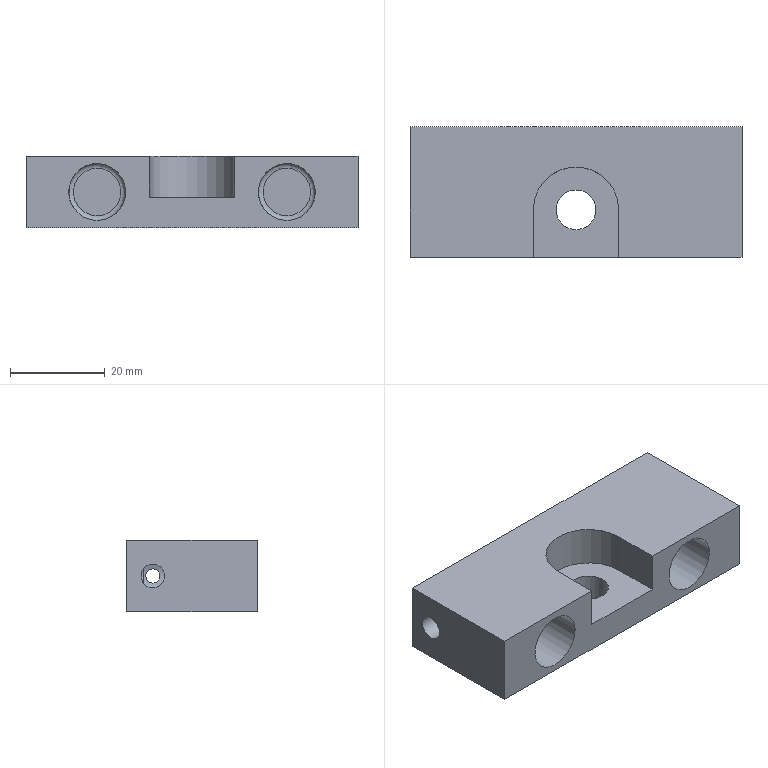NC program | NX | posted with a generic post | part box 70 x 27.5 x 15 mm
Lines 3562 to 3781 of 3781:
(PLANAR_MILL_8_COPY , TOOL : D8R1)
N7098 T04 M6
N7100 G54
N7102 G17 G0 G90 X-19.087 Y1.24 B0. C0. S2500 M3
N7104 G43 Z20. H4
N7106 Z-5.983 B-180. C-180.
N7108 G94 G1 Z-7.983 F300.
N7110 G41 X-19. Y1.732 D4
N7112 Y2.
N7114 G3 X-20. Y3. R1.
N7116 X-23. Y0. R3.
N7118 X-20. Y3. R-3.
N7120 X-21. Y2. R1.
N7122 G40
N7124 G1 X-20.913 Y1.508
N7126 X-19.087
N7128 G41 X-19. Y2.
N7130 G3 X-20. Y3. R1.
N7132 X-23. Y0. R3.
N7134 X-20. Y3. R-3.
N7136 X-21. Y2. R1.
N7138 G1 Y1.732
N7140 G40
N7142 X-20.913 Y1.24
N7144 Z-5.983
N7146 G0 Z20.
N7148 X-19.087
N7150 Z-13.967
N7152 G1 Z-15.967
N7154 G41 X-19. Y1.732
N7156 Y2.
N7158 G3 X-20. Y3. R1.
N7160 X-23. Y0. R3.
N7162 X-20. Y3. R-3.
N7164 X-21. Y2. R1.
N7166 G40
N7168 G1 X-20.913 Y1.508
N7170 X-19.087
N7172 G41 X-19. Y2.
N7174 G3 X-20. Y3. R1.
N7176 X-23. Y0. R3.
N7178 X-20. Y3. R-3.
N7180 X-21. Y2. R1.
N7182 G1 Y1.732
N7184 G40
N7186 X-20.913 Y1.24
N7188 Z-13.967
N7190 G0 Z20.
N7192 X-19.087
N7194 Z-21.95
N7196 G1 Z-23.95
N7198 G41 X-19. Y1.732
N7200 Y2.
N7202 G3 X-20. Y3. R1.
N7204 X-23. Y0. R3.
N7206 X-20. Y3. R-3.
N7208 X-21. Y2. R1.
N7210 G40
N7212 G1 X-20.913 Y1.508
N7214 X-19.087
N7216 G41 X-19. Y2.
N7218 G3 X-20. Y3. R1.
N7220 X-23. Y0. R3.
N7222 X-20. Y3. R-3.
N7224 X-21. Y2. R1.
N7226 G1 Y1.732
N7228 G40
N7230 X-20.913 Y1.24
N7232 Z-21.95
N7234 G0 Z20.
N7236 X20.913
N7238 Z-5.983
N7240 G1 Z-7.983
N7242 G41 X21. Y1.732
N7244 Y2.
N7246 G3 X20. Y3. R1.
N7248 X17. Y0. R3.
N7250 X20. Y3. R-3.
N7252 X19. Y2. R1.
N7254 G40
N7256 G1 X19.087 Y1.508
N7258 X20.913
N7260 G41 X21. Y2.
N7262 G3 X20. Y3. R1.
N7264 X17. Y0. R3.
N7266 X20. Y3. R-3.
N7268 X19. Y2. R1.
N7270 G1 Y1.732
N7272 G40
N7274 X19.087 Y1.24
N7276 Z-5.983
N7278 G0 Z20.
N7280 X20.913
N7282 Z-13.967
N7284 G1 Z-15.967
N7286 G41 X21. Y1.732
N7288 Y2.
N7290 G3 X20. Y3. R1.
N7292 X17. Y0. R3.
N7294 X20. Y3. R-3.
N7296 X19. Y2. R1.
N7298 G40
N7300 G1 X19.087 Y1.508
N7302 X20.913
N7304 G41 X21. Y2.
N7306 G3 X20. Y3. R1.
N7308 X17. Y0. R3.
N7310 X20. Y3. R-3.
N7312 X19. Y2. R1.
N7314 G1 Y1.732
N7316 G40
N7318 X19.087 Y1.24
N7320 Z-13.967
N7322 G0 Z20.
N7324 X20.913
N7326 Z-21.95
N7328 G1 Z-23.95
N7330 G41 X21. Y1.732
N7332 Y2.
N7334 G3 X20. Y3. R1.
N7336 X17. Y0. R3.
N7338 X20. Y3. R-3.
N7340 X19. Y2. R1.
N7342 G40
N7344 G1 X19.087 Y1.508
N7346 X20.913
N7348 G41 X21. Y2.
N7350 G3 X20. Y3. R1.
N7352 X17. Y0. R3.
N7354 X20. Y3. R-3.
N7356 X19. Y2. R1.
N7358 G1 Y1.732
N7360 G40
N7362 X19.087 Y1.24
N7364 Z-21.95
N7366 G0 Z20.
(PLANAR_MILL_9 , TOOL : D8R1)
N7368 X-19.629 Y0.149 S3000
N7370 Z-23.
N7372 G1 Z-25.
N7374 G41 X-19. Y0.4
N7376 G3 X-20. Y1.4 R1.
N7378 X-21.4 Y0. R1.4
N7380 X-20. Y1.4 R-1.4
N7382 X-21. Y0.4 R1.
N7384 G40
N7386 G1 X-20.983 Y0.302
N7388 X-19.017 Y1.902
N7390 G41 X-19. Y2.
N7392 G3 X-20. Y3. R1.
N7394 X-23. Y0. R3.
N7396 X-20. Y3. R-3.
N7398 X-21. Y2. R1.
N7400 G1 Y1.732
N7402 G40
N7404 X-20.983 Y1.634
N7406 Z-23.
N7408 G0 Z20.
N7410 X20.371 Y0.149
N7412 Z-23.
N7414 G1 Z-25.
N7416 G41 X21. Y0.4
N7418 G3 X20. Y1.4 R1.
N7420 X18.6 Y0. R1.4
N7422 X20. Y1.4 R-1.4
N7424 X19. Y0.4 R1.
N7426 G40
N7428 G1 X19.017 Y0.302
N7430 X20.983 Y1.902
N7432 G41 X21. Y2.
N7434 G3 X20. Y3. R1.
N7436 X17. Y0. R3.
N7438 X20. Y3. R-3.
N7440 X19. Y2. R1.
N7442 G1 Y1.732
N7444 G40
N7446 X19.017 Y1.634
N7448 Z-23.
N7450 G0 Z20.
N7452 M5
(PLANAR_MILL_9_COPY , TOOL : 倒角D4-90度)
N7454 T05 M6
N7456 G54
N7458 G17 G0 G90 X-19.017 Y3.36 B0. C0. S3000 M3
N7460 G43 Z20. H5
N7462 Z0.5 B-180. C-180.
N7464 G94 G1 Z-1.5 F300.
N7466 G41 X-19. Y3.458 D5
N7468 Y3.6
N7470 G3 X-20. Y4.6 R1.
N7472 X-24.6 Y0. R4.6
N7474 X-20. Y4.6 R-4.6
N7476 X-21. Y3.6 R1.
N7478 G1 Y3.458
N7480 G40
N7482 X-20.983 Y3.36
N7484 Z0.5
N7486 G0 Z20.
N7488 X20.983
N7490 Z0.5
N7492 G1 Z-1.5
N7494 G41 X21. Y3.458
N7496 Y3.6
N7498 G3 X20. Y4.6 R1.
N7500 X15.4 Y0. R4.6
N7502 X20. Y4.6 R-4.6
N7504 X19. Y3.6 R1.
N7506 G1 Y3.458
N7508 G40
N7510 X19.017 Y3.36
N7512 Z0.5
N7514 G0 Z20.
N7516 M5
N7518 M2